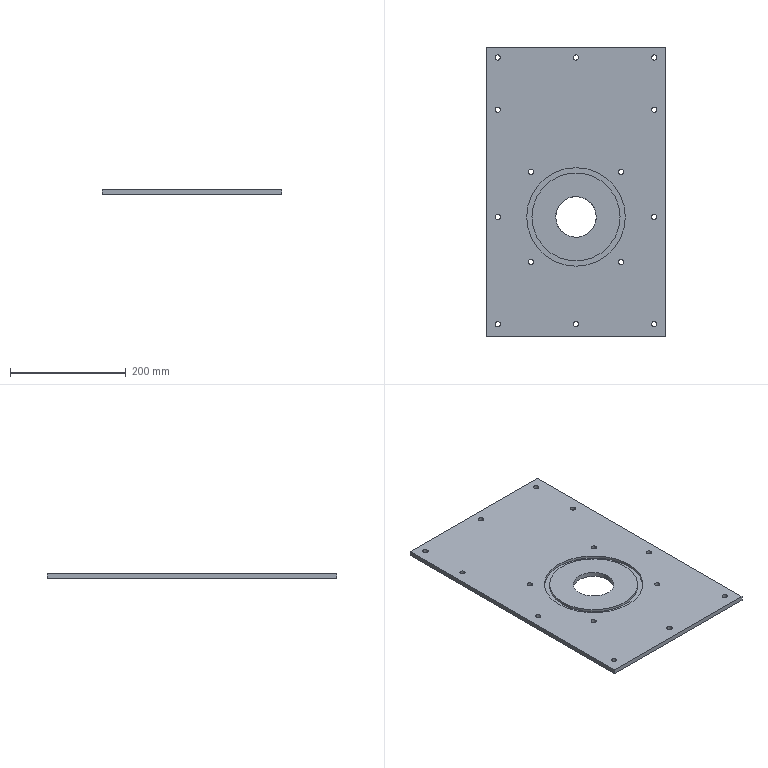Part | STEP file | 101000007717 | 1 solid | 42 faces | box 310 x 500 x 8 mm | volume 1181603 mm3 | cylinder 34 | plane 8 | commonest cylinder face diameters 9 x28 70 x2 152 x2 170 x2